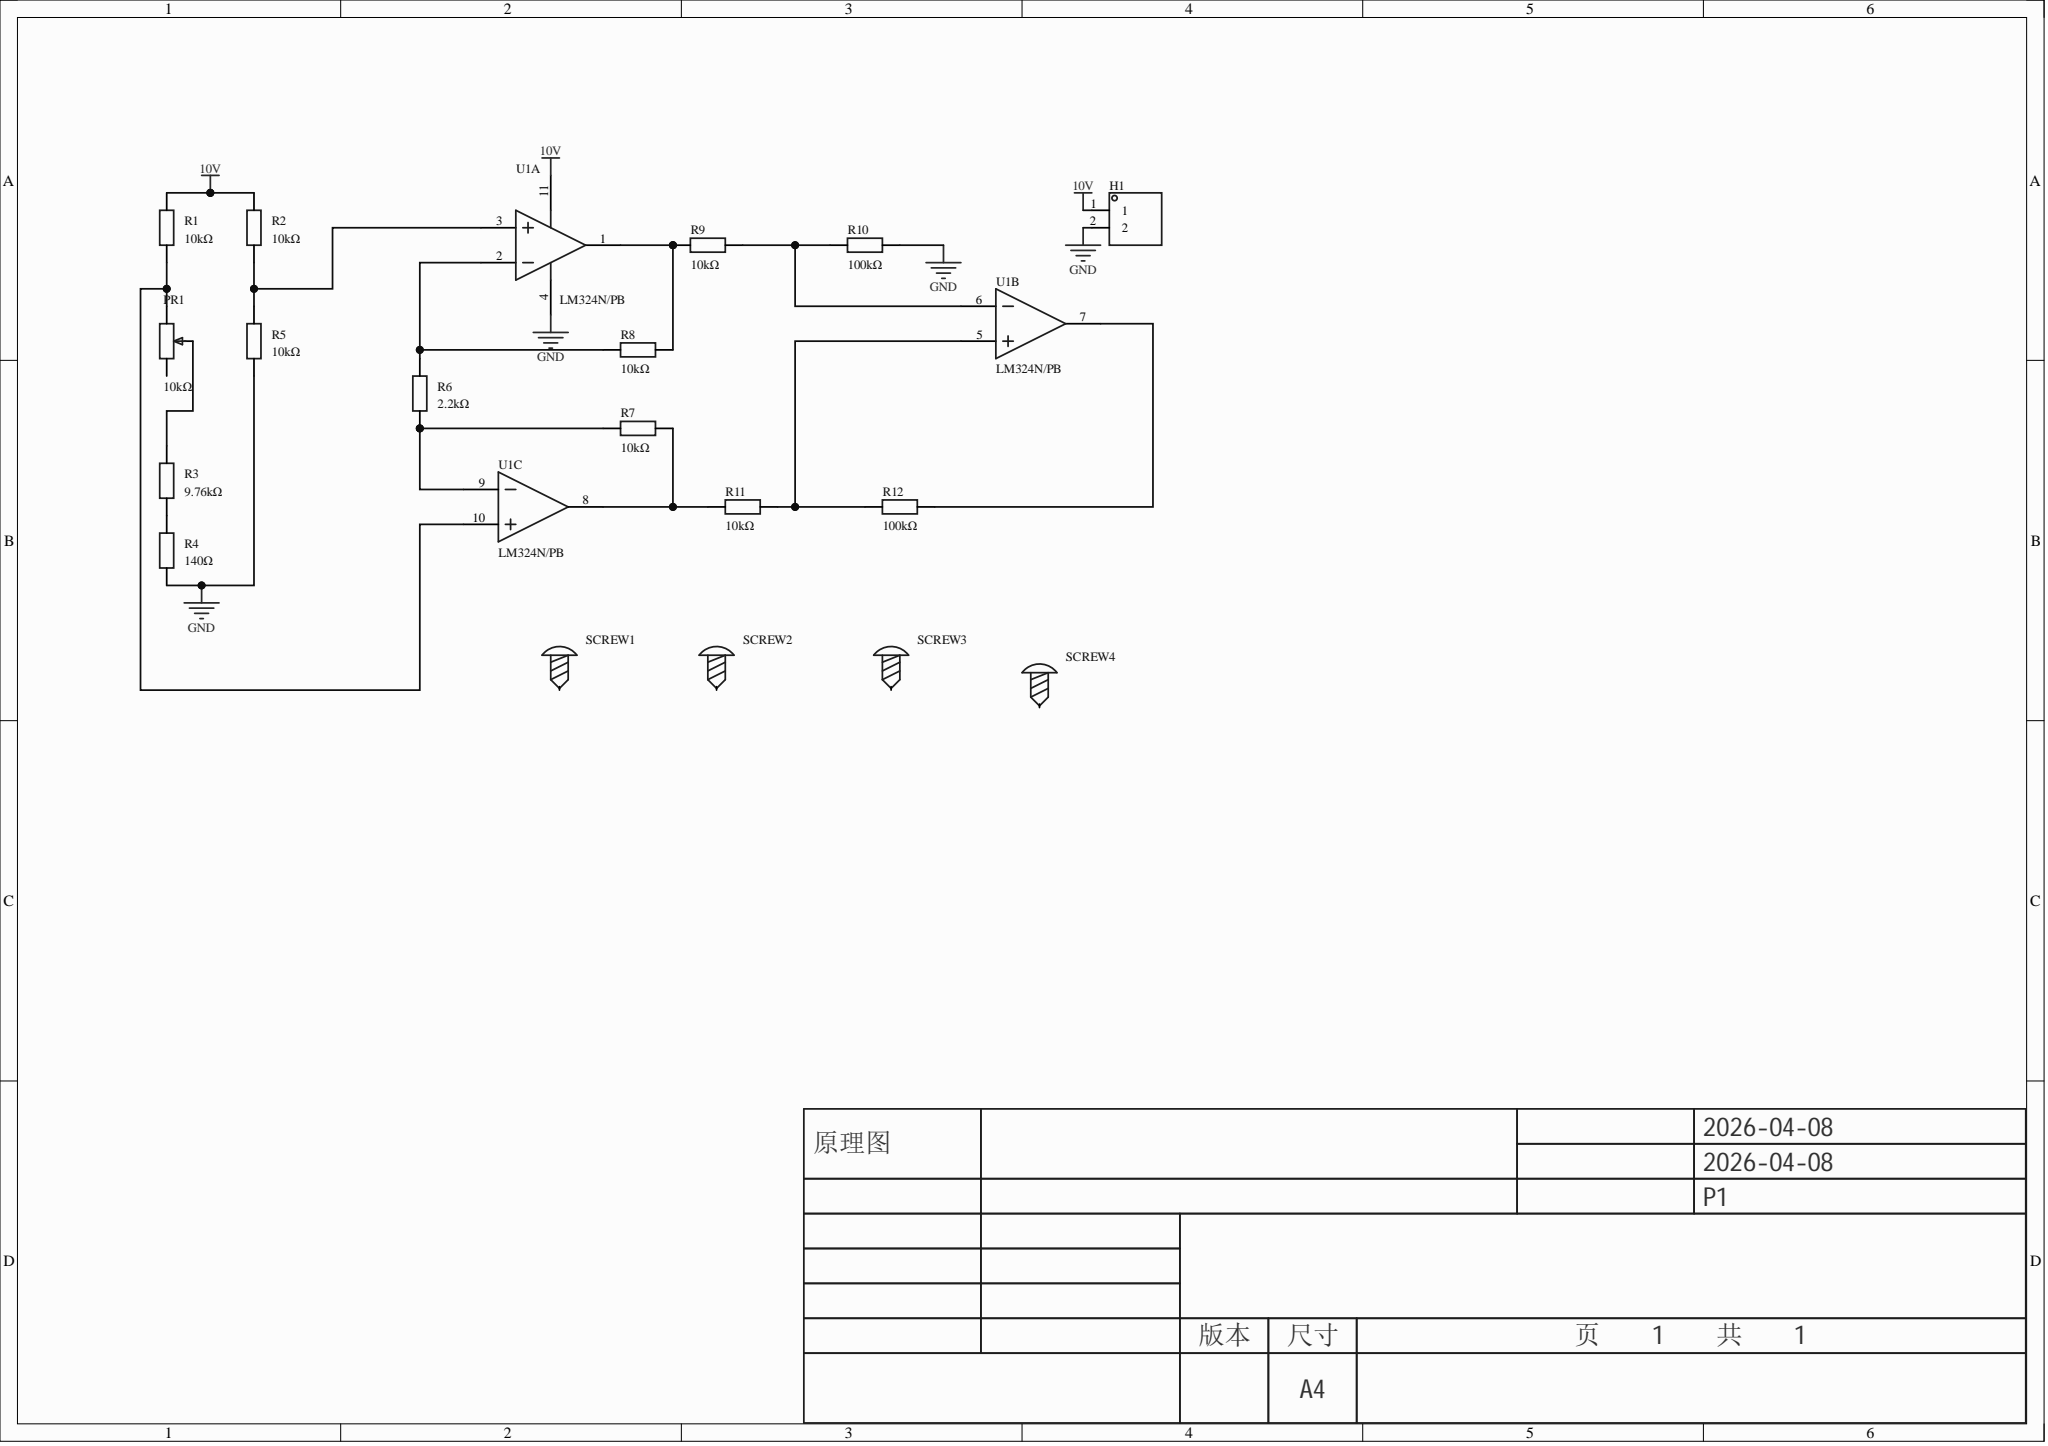Circuit board | Altium Designer | 19 parts | 13 nets
Bill of materials:
Comment,Description,Designator,Footprint,LibRef,Quantity
"","","H1","HDR-TH_2P-P2.54-V-M-1","HDR-M_2.54_1x2P","1"
"10kΩ","","PR1","R_3296","R_3296","1"
"10kΩ","","R1, R2, R5, R7, R8, R9, R11","Res_1/8W","Res_AXIAL-1/8W","7"
"9.76kΩ","","R3","Res_1/8W","Res_AXIAL-1/8W","1"
"140Ω","","R4","Res_1/8W","Res_AXIAL-1/8W","1"
"2.2kΩ","","R6","Res_1/8W","Res_AXIAL-1/8W","1"
"100kΩ","","R10, R12","Res_1/8W","Res_AXIAL-1/8W","2"
"","","SCREW1, SCREW2, SCREW3, SCREW4","M2螺丝","M2螺丝","4"
"LM324N/PB","放大器数:4;轨到轨:-;增益带宽积(GBW):-;输入失调电压(Vos):2mV;压摆率(SR):-;输入偏置电流(Ib):45nA;","U1","PDIP-14_L19.2-W6.6-P2.54-LS7.6-BL","LM324N/PB","1"
Netlist (Protel format):
[
H1
HDR-TH_2P-P2.54-V-M-1




]
[
PR1
R_3296
10kΩ



]
[
R1
Res_1/8W
10kΩ



]
[
R2
Res_1/8W
10kΩ



]
[
R3
Res_1/8W
9.76kΩ



]
[
R4
Res_1/8W
140Ω



]
[
R5
Res_1/8W
10kΩ



]
[
R6
Res_1/8W
2.2kΩ



]
[
R7
Res_1/8W
10kΩ



]
[
R8
Res_1/8W
10kΩ



]
[
R9
Res_1/8W
10kΩ



]
[
R10
Res_1/8W
100kΩ



]
[
R11
Res_1/8W
10kΩ



]
[
R12
Res_1/8W
100kΩ



]
[
SCREW1
M2螺丝




]
[
SCREW2
M2螺丝




]
[
SCREW3
M2螺丝




]
[
SCREW4
M2螺丝




]
[
U1
PDIP-14_L19.2-W6.6-P2.54-LS7.6-BL
LM324N/PB



]
(
NetR12_1
R12-1
U1-7
)
(
NetR11_1
R11-1
R12-2
U1-5
)
(
NetR9_1
R9-1
R10-2
U1-6
)
(
NetR8_1
R8-1
R9-2
U1-1
)
(
NetR7_1
R7-1
R11-2
U1-8
)
(
NetR6_2
R6-2
R8-2
U1-2
)
(
NetR6_1
R6-1
R7-2
U1-9
)
(
NetR3_1
R3-1
R4-2
)
(
NetR2_1
R2-1
R5-2
U1-3
)
(
NetPR1_3
PR1-3
R1-1
U1-10
)
(
NetPR1_2
PR1-2
R3-2
)
(
GND
H1-2
R4-1
R5-1
R10-1
U1-4
)
(
10V
H1-1
R1-2
R2-2
U1-11
)